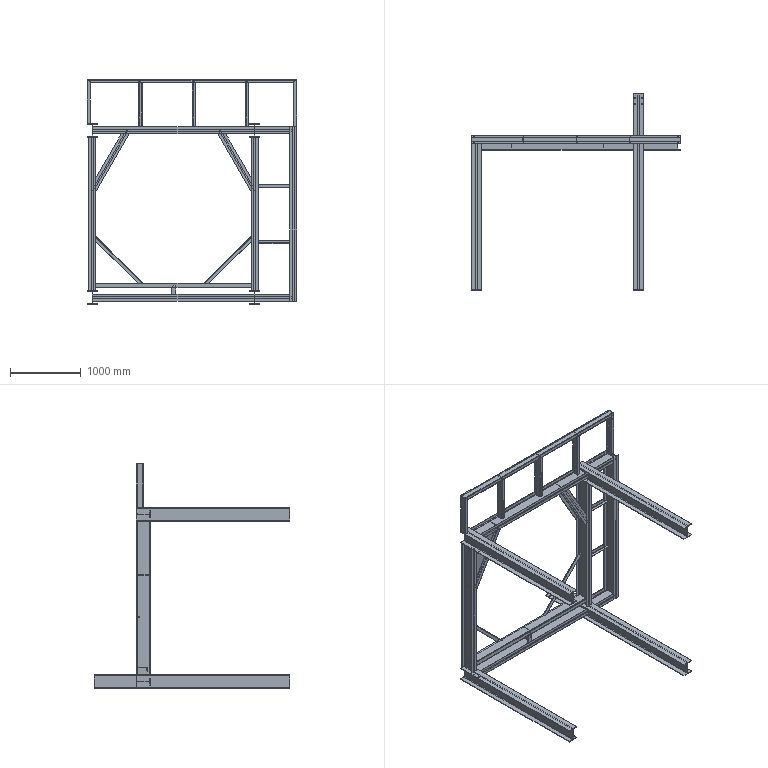Part | STEP file | Transfer kettle bracket 9 body_Default<As Machined> | 27 solids | 544 faces | box 2975 x 2778 x 3187 mm | volume 87808085 mm3 | plane 415 | cylinder 129 | commonest cylinder face diameters 16 x52 19 x24 8.4 x12 17 x12 2.66 x10 10 x4